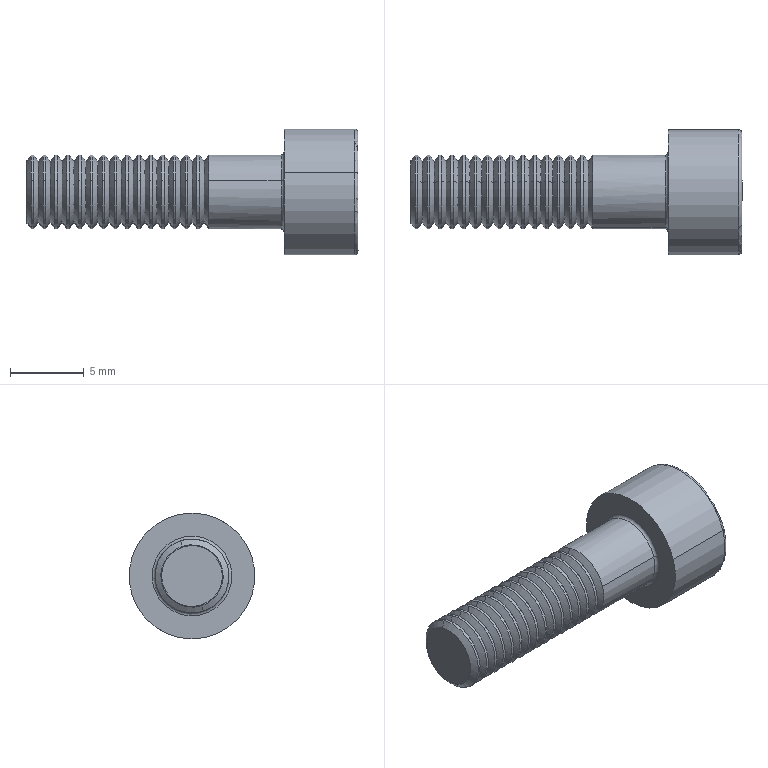Part | STEP file | Socket Head Cap Screw_ISO(ISO 4762 M5 x 20 --- 20S)-128_Valor predeterminado | 1 solid | 119 faces | box 22.439 x 8.5 x 8.5 mm | volume 552.666 mm3 | cone 66 | cylinder 34 | plane 15 | torus 4 | commonest cylinder face diameters 5 x32 8.5 x2